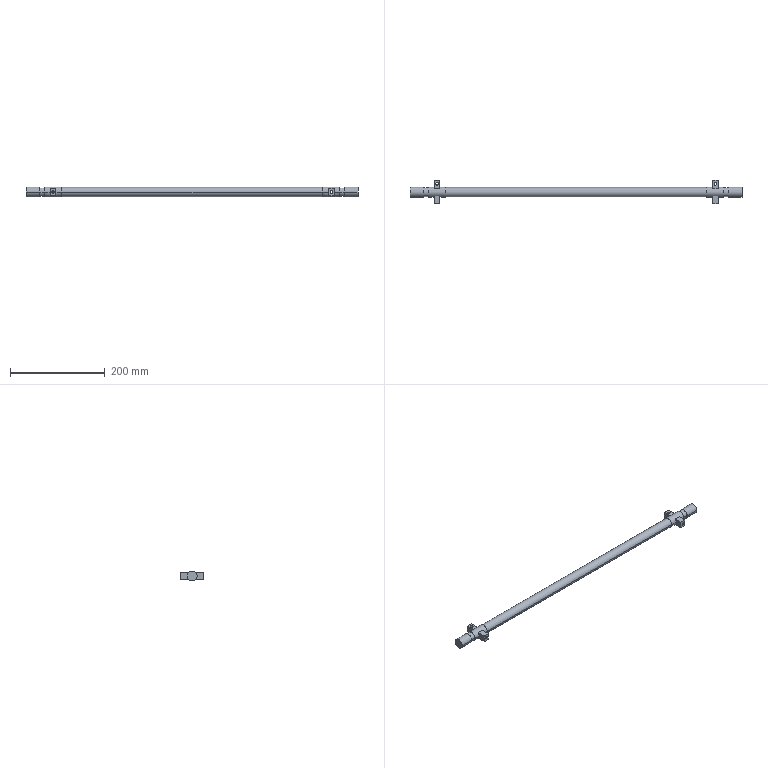Part | SolidWorks | features HoleWzd 2, ICE 2, LPattern 1, Revolution 1 | 1 solid | 58 faces | box 700 x 50.5 x 21 mm | volume 231919 mm3 | cylinder 30 | plane 28 | commonest cylinder face diameters 5.5 x16 21 x8 19 x4 20 x2